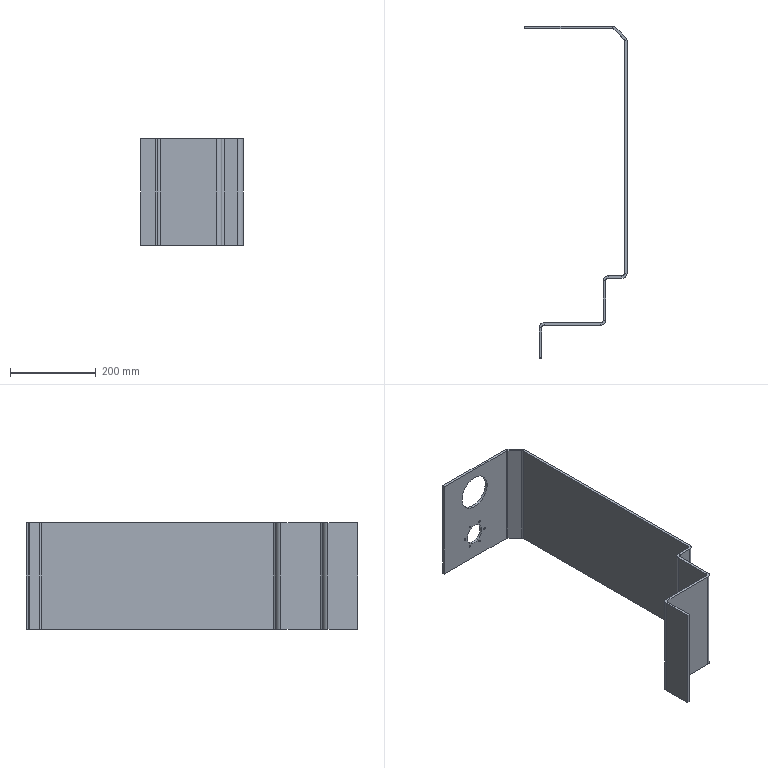Part | SolidWorks | features FlatPattern 1, HoleWzd 1, ICE 1, SMBaseFlange 1, SheetMetal 1 | 1 solid | 70 faces | box 239 x 776 x 250 mm | volume 1720525 mm3 | plane 42 | cylinder 28 | commonest cylinder face diameters 4.2 x12 12 x6 24 x6 48 x2 83 x2